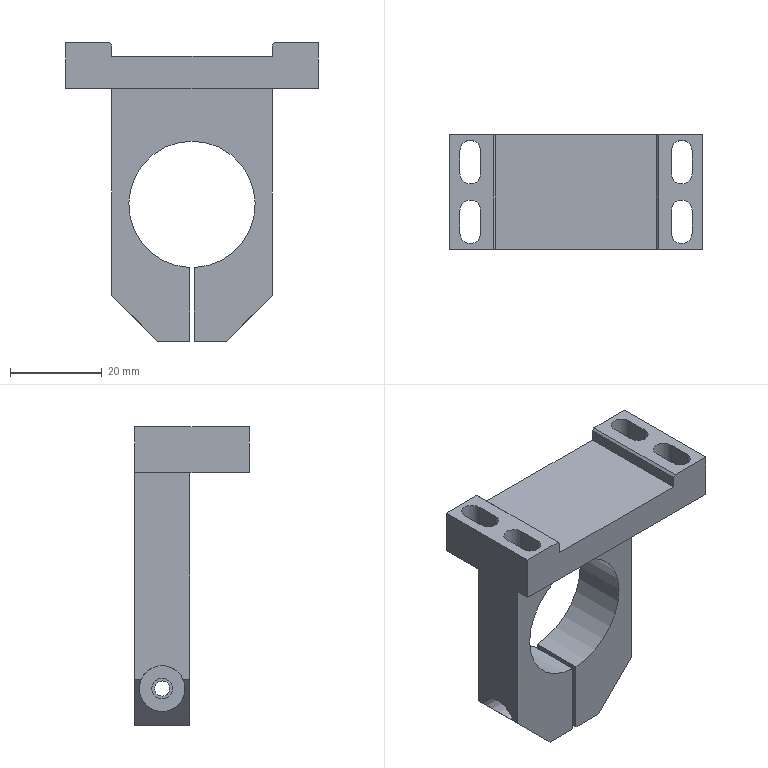Part | SolidWorks | features ICE 6, Chamfer 2, Extrusion 1, HoleWzd 1 | 1 solid | 45 faces | box 55 x 25 x 65 mm | volume 23319 mm3 | plane 30 | cylinder 15 | commonest cylinder face diameters 4.5 x10 3.3 x2 10 x2 27.5 x1
STEP:
#1=CARTESIAN_POINT('',(17.15,6.,-20.15));
#2=VERTEX_POINT('',#1);
#3=CARTESIAN_POINT('',(13.85,6.,-23.45));
#4=VERTEX_POINT('',#3);
#5=CARTESIAN_POINT('',(17.15,6.,-20.15));
#6=CARTESIAN_POINT('',(17.15,2.7,-20.15));
#7=CARTESIAN_POINT('',(13.85,2.7,-23.45));
#8=CARTESIAN_POINT('',(13.85,6.,-23.45));
#9=(BOUNDED_CURVE()B_SPLINE_CURVE(3,(#5,#6,#7,#8),.UNSPECIFIED.,.F.,.F.)B_SPLINE_CURVE_WITH_KNOTS((4,4),(3.142,6.283),.UNSPECIFIED.)CURVE()GEOMETRIC_REPRESENTATION_ITEM()RATIONAL_B_SPLINE_CURVE((1.,0.3333,0.3333,1.))REPRESENTATION_ITEM(''));
#10=EDGE_CURVE('',#2,#4,#9,.T.);
#11=ORIENTED_EDGE('',*,*,#10,.T.);
#12=CARTESIAN_POINT('',(0.5,6.,-23.45));
#13=VERTEX_POINT('',#12);
#14=CARTESIAN_POINT('',(0.5,6.,-23.45));
#15=DIRECTION('',(-1.,0.,0.));
#16=VECTOR('',#15,1000.);
#17=LINE('',#14,#16);
#18=EDGE_CURVE('',#4,#13,#17,.T.);
#19=ORIENTED_EDGE('',*,*,#18,.T.);
#20=CARTESIAN_POINT('',(0.5,6.,-20.15));
#21=VERTEX_POINT('',#20);
#22=CARTESIAN_POINT('',(0.5,6.,-21.8));
#23=DIRECTION('',(-1.,0.,0.));
#24=DIRECTION('',(0.,0.,1.));
#25=AXIS2_PLACEMENT_3D('',#22,#23,#24);
#26=CIRCLE('',#25,1.65);
#27=EDGE_CURVE('',#13,#21,#26,.T.);
#28=ORIENTED_EDGE('',*,*,#27,.T.);
#29=CARTESIAN_POINT('',(0.5,6.,-20.15));
#30=DIRECTION('',(-1.,0.,0.));
#31=VECTOR('',#30,1000.);
#32=LINE('',#29,#31);
#33=EDGE_CURVE('',#2,#21,#32,.T.);
#34=ORIENTED_EDGE('',*,*,#33,.F.);
#35=EDGE_LOOP('',(#11,#19,#28,#34));
#36=FACE_OUTER_BOUND('',#35,.T.);
#37=CARTESIAN_POINT('',(0.5,6.,-21.8));
#38=DIRECTION('',(-1.,0.,0.));
#39=DIRECTION('',(0.,0.,1.));
#40=AXIS2_PLACEMENT_3D('',#37,#38,#39);
#41=CYLINDRICAL_SURFACE('',#40,1.65);
#42=ADVANCED_FACE('',(#36),#41,.F.);
#43=CARTESIAN_POINT('',(-0.5,6.,-19.55));
#44=VERTEX_POINT('',#43);
#45=CARTESIAN_POINT('',(-0.5,6.,-24.05));
#46=VERTEX_POINT('',#45);
#47=CARTESIAN_POINT('',(-0.5,6.,-21.8));
#48=DIRECTION('',(1.,0.,0.));
#49=DIRECTION('',(0.,0.,1.));
#50=AXIS2_PLACEMENT_3D('',#47,#48,#49);
#51=CIRCLE('',#50,2.25);
#52=EDGE_CURVE('',#44,#46,#51,.T.);
#53=ORIENTED_EDGE('',*,*,#52,.T.);
#54=CARTESIAN_POINT('',(-7.5,6.,-24.05));
#55=VERTEX_POINT('',#54);
#56=CARTESIAN_POINT('',(5.864,6.,-24.05));
#57=DIRECTION('',(-1.,0.,0.));
#58=VECTOR('',#57,1000.);
#59=LINE('',#56,#58);
#60=EDGE_CURVE('',#46,#55,#59,.T.);
#61=ORIENTED_EDGE('',*,*,#60,.T.);
#62=CARTESIAN_POINT('',(-7.5,6.,-19.55));
#63=VERTEX_POINT('',#62);
#64=CARTESIAN_POINT('',(-7.5,6.,-21.8));
#65=DIRECTION('',(-1.,0.,0.));
#66=DIRECTION('',(0.,0.,1.));
#67=AXIS2_PLACEMENT_3D('',#64,#65,#66);
#68=CIRCLE('',#67,2.25);
#69=EDGE_CURVE('',#55,#63,#68,.T.);
#70=ORIENTED_EDGE('',*,*,#69,.T.);
#71=CARTESIAN_POINT('',(5.864,6.,-19.55));
#72=DIRECTION('',(-1.,0.,0.));
#73=VECTOR('',#72,1000.);
#74=LINE('',#71,#73);
#75=EDGE_CURVE('',#44,#63,#74,.T.);
#76=ORIENTED_EDGE('',*,*,#75,.F.);
#77=EDGE_LOOP('',(#53,#61,#70,#76));
#78=FACE_OUTER_BOUND('',#77,.T.);
#79=CARTESIAN_POINT('',(5.864,6.,-21.8));
#80=DIRECTION('',(-1.,0.,0.));
#81=DIRECTION('',(0.,0.,1.));
#82=AXIS2_PLACEMENT_3D('',#79,#80,#81);
#83=CYLINDRICAL_SURFACE('',#82,2.25);
#84=ADVANCED_FACE('',(#78),#83,.F.);
#85=CARTESIAN_POINT('',(-7.5,6.,-26.8));
#86=VERTEX_POINT('',#85);
#87=CARTESIAN_POINT('',(-7.5,6.,-16.8));
#88=VERTEX_POINT('',#87);
#89=CARTESIAN_POINT('',(-7.5,6.,-21.8));
#90=DIRECTION('',(-1.,0.,0.));
#91=DIRECTION('',(0.,0.,1.));
#92=AXIS2_PLACEMENT_3D('',#89,#90,#91);
#93=CIRCLE('',#92,5.);
#94=EDGE_CURVE('',#86,#88,#93,.T.);
#95=ORIENTED_EDGE('',*,*,#94,.F.);
#96=CARTESIAN_POINT('',(-10.5,6.,-26.8));
#97=VERTEX_POINT('',#96);
#98=CARTESIAN_POINT('',(-7.5,6.,-26.8));
#99=DIRECTION('',(-1.,0.,0.));
#100=VECTOR('',#99,1000.);
#101=LINE('',#98,#100);
#102=EDGE_CURVE('',#86,#97,#101,.T.);
#103=ORIENTED_EDGE('',*,*,#102,.T.);
#104=CARTESIAN_POINT('',(-17.5,1.417,-19.8));
#105=VERTEX_POINT('',#104);
#106=CARTESIAN_POINT('',(-10.5,6.,-26.8));
#107=CARTESIAN_POINT('',(-10.5,2.007,-26.8));
#108=CARTESIAN_POINT('',(-13.841,-0.1797,-23.459));
#109=CARTESIAN_POINT('',(-17.5,1.417,-19.8));
#110=(BOUNDED_CURVE()B_SPLINE_CURVE(3,(#106,#107,#108,#109),.UNSPECIFIED.,.F.,.F.)B_SPLINE_CURVE_WITH_KNOTS((4,4),(3.142,5.124),.UNSPECIFIED.)CURVE()GEOMETRIC_REPRESENTATION_ITEM()RATIONAL_B_SPLINE_CURVE((1.,0.6985,0.6985,1.))REPRESENTATION_ITEM(''));
#111=EDGE_CURVE('',#97,#105,#110,.T.);
#112=ORIENTED_EDGE('',*,*,#111,.T.);
#113=CARTESIAN_POINT('',(-17.5,6.,-16.8));
#114=VERTEX_POINT('',#113);
#115=CARTESIAN_POINT('',(-17.5,6.,-21.8));
#116=DIRECTION('',(-1.,0.,0.));
#117=DIRECTION('',(0.,0.,1.));
#118=AXIS2_PLACEMENT_3D('',#115,#116,#117);
#119=CIRCLE('',#118,5.);
#120=EDGE_CURVE('',#105,#114,#119,.T.);
#121=ORIENTED_EDGE('',*,*,#120,.T.);
#122=CARTESIAN_POINT('',(-7.5,6.,-16.8));
#123=DIRECTION('',(-1.,0.,0.));
#124=VECTOR('',#123,1000.);
#125=LINE('',#122,#124);
#126=EDGE_CURVE('',#88,#114,#125,.T.);
#127=ORIENTED_EDGE('',*,*,#126,.F.);
#128=EDGE_LOOP('',(#95,#103,#112,#121,#127));
#129=FACE_OUTER_BOUND('',#128,.T.);
#130=CARTESIAN_POINT('',(-7.5,6.,-21.8));
#131=DIRECTION('',(-1.,0.,0.));
#132=DIRECTION('',(0.,0.,1.));
#133=AXIS2_PLACEMENT_3D('',#130,#131,#132);
#134=CYLINDRICAL_SURFACE('',#133,5.);
#135=ADVANCED_FACE('',(#129),#134,.F.);
#136=CARTESIAN_POINT('',(7.5,0.,-29.8));
#137=VERTEX_POINT('',#136);
#138=CARTESIAN_POINT('',(0.5,0.,-29.8));
#139=VERTEX_POINT('',#138);
#140=CARTESIAN_POINT('',(-17.5,0.,-29.8));
#141=DIRECTION('',(-1.,0.,0.));
#142=VECTOR('',#141,1000.);
#143=LINE('',#140,#142);
#144=EDGE_CURVE('',#137,#139,#143,.T.);
#145=ORIENTED_EDGE('',*,*,#144,.T.);
#146=CARTESIAN_POINT('',(0.5,12.,-29.8));
#147=VERTEX_POINT('',#146);
#148=CARTESIAN_POINT('',(0.5,12.,-29.8));
#149=DIRECTION('',(0.,1.,0.));
#150=VECTOR('',#149,1000.);
#151=LINE('',#148,#150);
#152=EDGE_CURVE('',#139,#147,#151,.T.);
#153=ORIENTED_EDGE('',*,*,#152,.T.);
#154=CARTESIAN_POINT('',(7.5,12.,-29.8));
#155=VERTEX_POINT('',#154);
#156=CARTESIAN_POINT('',(-17.5,12.,-29.8));
#157=DIRECTION('',(-1.,0.,0.));
#158=VECTOR('',#157,1000.);
#159=LINE('',#156,#158);
#160=EDGE_CURVE('',#155,#147,#159,.T.);
#161=ORIENTED_EDGE('',*,*,#160,.F.);
#162=CARTESIAN_POINT('',(7.5,12.,-29.8));
#163=DIRECTION('',(0.,-1.,0.));
#164=VECTOR('',#163,1000.);
#165=LINE('',#162,#164);
#166=EDGE_CURVE('',#155,#137,#165,.T.);
#167=ORIENTED_EDGE('',*,*,#166,.T.);
#168=EDGE_LOOP('',(#145,#153,#161,#167));
#169=FACE_OUTER_BOUND('',#168,.T.);
#170=CARTESIAN_POINT('',(-17.5,12.,-29.8));
#171=DIRECTION('',(0.,0.,1.));
#172=DIRECTION('',(1.,0.,0.));
#173=AXIS2_PLACEMENT_3D('',#170,#171,#172);
#174=PLANE('',#173);
#175=ADVANCED_FACE('',(#169),#174,.F.);
#176=CARTESIAN_POINT('',(25.25,-4.5,35.2));
#177=VERTEX_POINT('',#176);
#178=CARTESIAN_POINT('',(25.25,-9.5,35.2));
#179=VERTEX_POINT('',#178);
#180=CARTESIAN_POINT('',(25.25,12.,35.2));
#181=DIRECTION('',(0.,-1.,0.));
#182=VECTOR('',#181,1000.);
#183=LINE('',#180,#182);
#184=EDGE_CURVE('',#177,#179,#183,.T.);
#185=ORIENTED_EDGE('',*,*,#184,.T.);
#186=CARTESIAN_POINT('',(20.75,-9.5,35.2));
#187=VERTEX_POINT('',#186);
#188=CARTESIAN_POINT('',(23.,-9.5,35.2));
#189=DIRECTION('',(0.,0.,-1.));
#190=DIRECTION('',(-1.,0.,0.));
#191=AXIS2_PLACEMENT_3D('',#188,#189,#190);
#192=CIRCLE('',#191,2.25);
#193=EDGE_CURVE('',#179,#187,#192,.T.);
#194=ORIENTED_EDGE('',*,*,#193,.T.);
#195=CARTESIAN_POINT('',(20.75,-4.5,35.2));
#196=VERTEX_POINT('',#195);
#197=CARTESIAN_POINT('',(20.75,12.,35.2));
#198=DIRECTION('',(0.,1.,0.));
#199=VECTOR('',#198,1000.);
#200=LINE('',#197,#199);
#201=EDGE_CURVE('',#187,#196,#200,.T.);
#202=ORIENTED_EDGE('',*,*,#201,.T.);
#203=CARTESIAN_POINT('',(23.,-4.5,35.2));
#204=DIRECTION('',(0.,0.,-1.));
#205=DIRECTION('',(-1.,0.,0.));
#206=AXIS2_PLACEMENT_3D('',#203,#204,#205);
#207=CIRCLE('',#206,2.25);
#208=EDGE_CURVE('',#196,#177,#207,.T.);
#209=ORIENTED_EDGE('',*,*,#208,.T.);
#210=EDGE_LOOP('',(#185,#194,#202,#209));
#211=FACE_BOUND('',#210,.T.);
#212=CARTESIAN_POINT('',(20.75,3.5,35.2));
#213=VERTEX_POINT('',#212);
#214=CARTESIAN_POINT('',(20.75,8.5,35.2));
#215=VERTEX_POINT('',#214);
#216=CARTESIAN_POINT('',(20.75,12.,35.2));
#217=DIRECTION('',(0.,1.,0.));
#218=VECTOR('',#217,1000.);
#219=LINE('',#216,#218);
#220=EDGE_CURVE('',#213,#215,#219,.T.);
#221=ORIENTED_EDGE('',*,*,#220,.T.);
#222=CARTESIAN_POINT('',(25.25,8.5,35.2));
#223=VERTEX_POINT('',#222);
#224=CARTESIAN_POINT('',(23.,8.5,35.2));
#225=DIRECTION('',(0.,0.,-1.));
#226=DIRECTION('',(-1.,0.,0.));
#227=AXIS2_PLACEMENT_3D('',#224,#225,#226);
#228=CIRCLE('',#227,2.25);
#229=EDGE_CURVE('',#215,#223,#228,.T.);
#230=ORIENTED_EDGE('',*,*,#229,.T.);
#231=CARTESIAN_POINT('',(25.25,3.5,35.2));
#232=VERTEX_POINT('',#231);
#233=CARTESIAN_POINT('',(25.25,12.,35.2));
#234=DIRECTION('',(0.,-1.,0.));
#235=VECTOR('',#234,1000.);
#236=LINE('',#233,#235);
#237=EDGE_CURVE('',#223,#232,#236,.T.);
#238=ORIENTED_EDGE('',*,*,#237,.T.);
#239=CARTESIAN_POINT('',(23.,3.5,35.2));
#240=DIRECTION('',(0.,0.,-1.));
#241=DIRECTION('',(-1.,0.,0.));
#242=AXIS2_PLACEMENT_3D('',#239,#240,#241);
#243=CIRCLE('',#242,2.25);
#244=EDGE_CURVE('',#232,#213,#243,.T.);
#245=ORIENTED_EDGE('',*,*,#244,.T.);
#246=EDGE_LOOP('',(#221,#230,#238,#245));
#247=FACE_BOUND('',#246,.T.);
#248=CARTESIAN_POINT('',(18.,12.,35.2));
#249=VERTEX_POINT('',#248);
#250=CARTESIAN_POINT('',(27.5,12.,35.2));
#251=VERTEX_POINT('',#250);
#252=CARTESIAN_POINT('',(-17.5,12.,35.2));
#253=DIRECTION('',(1.,0.,0.));
#254=VECTOR('',#253,1000.);
#255=LINE('',#252,#254);
#256=EDGE_CURVE('',#249,#251,#255,.T.);
#257=ORIENTED_EDGE('',*,*,#256,.F.);
#258=CARTESIAN_POINT('',(18.,-13.,35.2));
#259=VERTEX_POINT('',#258);
#260=CARTESIAN_POINT('',(18.,12.,35.2));
#261=DIRECTION('',(0.,-1.,0.));
#262=VECTOR('',#261,1000.);
#263=LINE('',#260,#262);
#264=EDGE_CURVE('',#249,#259,#263,.T.);
#265=ORIENTED_EDGE('',*,*,#264,.T.);
#266=CARTESIAN_POINT('',(27.5,-13.,35.2));
#267=VERTEX_POINT('',#266);
#268=CARTESIAN_POINT('',(-27.5,-13.,35.2));
#269=DIRECTION('',(1.,0.,0.));
#270=VECTOR('',#269,1000.);
#271=LINE('',#268,#270);
#272=EDGE_CURVE('',#259,#267,#271,.T.);
#273=ORIENTED_EDGE('',*,*,#272,.T.);
#274=CARTESIAN_POINT('',(27.5,-13.,35.2));
#275=DIRECTION('',(0.,1.,0.));
#276=VECTOR('',#275,1000.);
#277=LINE('',#274,#276);
#278=EDGE_CURVE('',#267,#251,#277,.T.);
#279=ORIENTED_EDGE('',*,*,#278,.T.);
#280=EDGE_LOOP('',(#257,#265,#273,#279));
#281=FACE_OUTER_BOUND('',#280,.T.);
#282=CARTESIAN_POINT('',(-17.5,12.,35.2));
#283=DIRECTION('',(0.,0.,-1.));
#284=DIRECTION('',(-1.,0.,0.));
#285=AXIS2_PLACEMENT_3D('',#282,#283,#284);
#286=PLANE('',#285);
#287=ADVANCED_FACE('',(#211,#247,#281),#286,.F.);
#288=ORIENTED_EDGE('',*,*,#160,.T.);
#289=CARTESIAN_POINT('',(0.5,12.,-13.741));
#290=VERTEX_POINT('',#289);
#291=CARTESIAN_POINT('',(0.5,12.,-48.692));
#292=DIRECTION('',(0.,0.,-1.));
#293=VECTOR('',#292,1000.);
#294=LINE('',#291,#293);
#295=EDGE_CURVE('',#290,#147,#294,.T.);
#296=ORIENTED_EDGE('',*,*,#295,.F.);
#297=CARTESIAN_POINT('',(-0.5,12.,-13.741));
#298=VERTEX_POINT('',#297);
#299=CARTESIAN_POINT('',(0.,12.,0.));
#300=DIRECTION('',(0.,1.,0.));
#301=DIRECTION('',(0.,0.,1.));
#302=AXIS2_PLACEMENT_3D('',#299,#300,#301);
#303=CIRCLE('',#302,13.75);
#304=EDGE_CURVE('',#298,#290,#303,.T.);
#305=ORIENTED_EDGE('',*,*,#304,.F.);
#306=CARTESIAN_POINT('',(-0.5,12.,-29.8));
#307=VERTEX_POINT('',#306);
#308=CARTESIAN_POINT('',(-0.5,12.,-48.692));
#309=DIRECTION('',(0.,0.,1.));
#310=VECTOR('',#309,1000.);
#311=LINE('',#308,#310);
#312=EDGE_CURVE('',#307,#298,#311,.T.);
#313=ORIENTED_EDGE('',*,*,#312,.F.);
#314=CARTESIAN_POINT('',(-7.5,12.,-29.8));
#315=VERTEX_POINT('',#314);
#316=CARTESIAN_POINT('',(-17.5,12.,-29.8));
#317=DIRECTION('',(-1.,0.,0.));
#318=VECTOR('',#317,1000.);
#319=LINE('',#316,#318);
#320=EDGE_CURVE('',#307,#315,#319,.T.);
#321=ORIENTED_EDGE('',*,*,#320,.T.);
#322=CARTESIAN_POINT('',(-17.5,12.,-19.8));
#323=VERTEX_POINT('',#322);
#324=CARTESIAN_POINT('',(-17.5,12.,-19.8));
#325=DIRECTION('',(-0.7071,0.,0.7071));
#326=VECTOR('',#325,1000.);
#327=LINE('',#324,#326);
#328=EDGE_CURVE('',#315,#323,#327,.T.);
#329=ORIENTED_EDGE('',*,*,#328,.T.);
#330=CARTESIAN_POINT('',(-17.5,12.,25.2));
#331=VERTEX_POINT('',#330);
#332=CARTESIAN_POINT('',(-17.5,12.,35.2));
#333=DIRECTION('',(0.,0.,1.));
#334=VECTOR('',#333,1000.);
#335=LINE('',#332,#334);
#336=EDGE_CURVE('',#323,#331,#335,.T.);
#337=ORIENTED_EDGE('',*,*,#336,.T.);
#338=CARTESIAN_POINT('',(-27.5,12.,25.2));
#339=VERTEX_POINT('',#338);
#340=CARTESIAN_POINT('',(-27.5,12.,25.2));
#341=DIRECTION('',(-1.,0.,0.));
#342=VECTOR('',#341,1000.);
#343=LINE('',#340,#342);
#344=EDGE_CURVE('',#331,#339,#343,.T.);
#345=ORIENTED_EDGE('',*,*,#344,.T.);
#346=CARTESIAN_POINT('',(-27.5,12.,35.2));
#347=VERTEX_POINT('',#346);
#348=CARTESIAN_POINT('',(-27.5,12.,25.2));
#349=DIRECTION('',(0.,0.,1.));
#350=VECTOR('',#349,1000.);
#351=LINE('',#348,#350);
#352=EDGE_CURVE('',#339,#347,#351,.T.);
#353=ORIENTED_EDGE('',*,*,#352,.T.);
#354=CARTESIAN_POINT('',(-18.,12.,35.2));
#355=VERTEX_POINT('',#354);
#356=CARTESIAN_POINT('',(-17.5,12.,35.2));
#357=DIRECTION('',(1.,0.,0.));
#358=VECTOR('',#357,1000.);
#359=LINE('',#356,#358);
#360=EDGE_CURVE('',#347,#355,#359,.T.);
#361=ORIENTED_EDGE('',*,*,#360,.T.);
#362=CARTESIAN_POINT('',(-17.5,12.,34.7));
#363=VERTEX_POINT('',#362);
#364=CARTESIAN_POINT('',(-18.,12.,35.2));
#365=DIRECTION('',(0.7071,0.,-0.7071));
#366=VECTOR('',#365,1000.);
#367=LINE('',#364,#366);
#368=EDGE_CURVE('',#355,#363,#367,.T.);
#369=ORIENTED_EDGE('',*,*,#368,.T.);
#370=CARTESIAN_POINT('',(-17.5,12.,32.2));
#371=VERTEX_POINT('',#370);
#372=CARTESIAN_POINT('',(-17.5,12.,38.2));
#373=DIRECTION('',(0.,0.,-1.));
#374=VECTOR('',#373,1000.);
#375=LINE('',#372,#374);
#376=EDGE_CURVE('',#363,#371,#375,.T.);
#377=ORIENTED_EDGE('',*,*,#376,.T.);
#378=CARTESIAN_POINT('',(17.5,12.,32.2));
#379=VERTEX_POINT('',#378);
#380=CARTESIAN_POINT('',(-17.5,12.,32.2));
#381=DIRECTION('',(1.,0.,0.));
#382=VECTOR('',#381,1000.);
#383=LINE('',#380,#382);
#384=EDGE_CURVE('',#371,#379,#383,.T.);
#385=ORIENTED_EDGE('',*,*,#384,.T.);
#386=CARTESIAN_POINT('',(17.5,12.,34.7));
#387=VERTEX_POINT('',#386);
#388=CARTESIAN_POINT('',(17.5,12.,38.2));
#389=DIRECTION('',(0.,0.,1.));
#390=VECTOR('',#389,1000.);
#391=LINE('',#388,#390);
#392=EDGE_CURVE('',#379,#387,#391,.T.);
#393=ORIENTED_EDGE('',*,*,#392,.T.);
#394=CARTESIAN_POINT('',(18.,12.,35.2));
#395=DIRECTION('',(0.7071,0.,0.7071));
#396=VECTOR('',#395,1000.);
#397=LINE('',#394,#396);
#398=EDGE_CURVE('',#387,#249,#397,.T.);
#399=ORIENTED_EDGE('',*,*,#398,.T.);
#400=ORIENTED_EDGE('',*,*,#256,.T.);
#401=CARTESIAN_POINT('',(27.5,12.,25.2));
#402=VERTEX_POINT('',#401);
#403=CARTESIAN_POINT('',(27.5,12.,25.2));
#404=DIRECTION('',(0.,0.,-1.));
#405=VECTOR('',#404,1000.);
#406=LINE('',#403,#405);
#407=EDGE_CURVE('',#251,#402,#406,.T.);
#408=ORIENTED_EDGE('',*,*,#407,.T.);
#409=CARTESIAN_POINT('',(17.5,12.,25.2));
#410=VERTEX_POINT('',#409);
#411=CARTESIAN_POINT('',(-27.5,12.,25.2));
#412=DIRECTION('',(-1.,0.,0.));
#413=VECTOR('',#412,1000.);
#414=LINE('',#411,#413);
#415=EDGE_CURVE('',#402,#410,#414,.T.);
#416=ORIENTED_EDGE('',*,*,#415,.T.);
#417=CARTESIAN_POINT('',(17.5,12.,-19.8));
#418=VERTEX_POINT('',#417);
#419=CARTESIAN_POINT('',(17.5,12.,35.2));
#420=DIRECTION('',(0.,0.,-1.));
#421=VECTOR('',#420,1000.);
#422=LINE('',#419,#421);
#423=EDGE_CURVE('',#410,#418,#422,.T.);
#424=ORIENTED_EDGE('',*,*,#423,.T.);
#425=CARTESIAN_POINT('',(7.5,12.,-29.8));
#426=DIRECTION('',(-0.7071,0.,-0.7071));
#427=VECTOR('',#426,1000.);
#428=LINE('',#425,#427);
#429=EDGE_CURVE('',#418,#155,#428,.T.);
#430=ORIENTED_EDGE('',*,*,#429,.T.);
#431=EDGE_LOOP('',(#288,#296,#305,#313,#321,#329,#337,#345,#353,#361,#369,#377,#385,#393,#399,#400,#408,#416,#424,#430));
#432=FACE_OUTER_BOUND('',#431,.T.);
#433=CARTESIAN_POINT('',(0.,12.,0.));
#434=DIRECTION('',(0.,-1.,0.));
#435=DIRECTION('',(0.,0.,-1.));
#436=AXIS2_PLACEMENT_3D('',#433,#434,#435);
#437=PLANE('',#436);
#438=ADVANCED_FACE('',(#432),#437,.F.);
#439=CARTESIAN_POINT('',(0.5,0.,-13.741));
#440=VERTEX_POINT('',#439);
#441=CARTESIAN_POINT('',(0.5,0.,0.));
#442=DIRECTION('',(0.,0.,1.));
#443=VECTOR('',#442,1000.);
#444=LINE('',#441,#443);
#445=EDGE_CURVE('',#139,#440,#444,.T.);
#446=ORIENTED_EDGE('',*,*,#445,.F.);
#447=ORIENTED_EDGE('',*,*,#144,.F.);
#448=CARTESIAN_POINT('',(17.5,0.,-19.8));
#449=VERTEX_POINT('',#448);
#450=CARTESIAN_POINT('',(18.65,0.,-18.65));
#451=DIRECTION('',(0.7071,0.,0.7071));
#452=VECTOR('',#451,1000.);
#453=LINE('',#450,#452);
#454=EDGE_CURVE('',#137,#449,#453,.T.);
#455=ORIENTED_EDGE('',*,*,#454,.T.);
#456=CARTESIAN_POINT('',(17.5,0.,25.2));
#457=VERTEX_POINT('',#456);
#458=CARTESIAN_POINT('',(17.5,0.,35.2));
#459=DIRECTION('',(0.,0.,-1.));
#460=VECTOR('',#459,1000.);
#461=LINE('',#458,#460);
#462=EDGE_CURVE('',#457,#449,#461,.T.);
#463=ORIENTED_EDGE('',*,*,#462,.F.);
#464=CARTESIAN_POINT('',(-17.5,0.,25.2));
#465=VERTEX_POINT('',#464);
#466=CARTESIAN_POINT('',(0.,0.,25.2));
#467=DIRECTION('',(1.,0.,0.));
#468=VECTOR('',#467,1000.);
#469=LINE('',#466,#468);
#470=EDGE_CURVE('',#465,#457,#469,.T.);
#471=ORIENTED_EDGE('',*,*,#470,.F.);
#472=CARTESIAN_POINT('',(-17.5,0.,-19.8));
#473=VERTEX_POINT('',#472);
#474=CARTESIAN_POINT('',(-17.5,0.,35.2));
#475=DIRECTION('',(0.,0.,1.));
#476=VECTOR('',#475,1000.);
#477=LINE('',#474,#476);
#478=EDGE_CURVE('',#473,#465,#477,.T.);
#479=ORIENTED_EDGE('',*,*,#478,.F.);
#480=CARTESIAN_POINT('',(-7.5,0.,-29.8));
#481=VERTEX_POINT('',#480);
#482=CARTESIAN_POINT('',(-18.65,0.,-18.65));
#483=DIRECTION('',(0.7071,0.,-0.7071));
#484=VECTOR('',#483,1000.);
#485=LINE('',#482,#484);
#486=EDGE_CURVE('',#473,#481,#485,.T.);
#487=ORIENTED_EDGE('',*,*,#486,.T.);
#488=CARTESIAN_POINT('',(-0.5,0.,-29.8));
#489=VERTEX_POINT('',#488);
#490=CARTESIAN_POINT('',(-17.5,0.,-29.8));
#491=DIRECTION('',(-1.,0.,0.));
#492=VECTOR('',#491,1000.);
#493=LINE('',#490,#492);
#494=EDGE_CURVE('',#489,#481,#493,.T.);
#495=ORIENTED_EDGE('',*,*,#494,.F.);
#496=CARTESIAN_POINT('',(-0.5,0.,-13.741));
#497=VERTEX_POINT('',#496);
#498=CARTESIAN_POINT('',(-0.5,0.,0.));
#499=DIRECTION('',(0.,0.,-1.));
#500=VECTOR('',#499,1000.);
#501=LINE('',#498,#500);
#502=EDGE_CURVE('',#497,#489,#501,.T.);
#503=ORIENTED_EDGE('',*,*,#502,.F.);
#504=CARTESIAN_POINT('',(0.,0.,0.));
#505=DIRECTION('',(0.,1.,0.));
#506=DIRECTION('',(0.,0.,1.));
#507=AXIS2_PLACEMENT_3D('',#504,#505,#506);
#508=CIRCLE('',#507,13.75);
#509=EDGE_CURVE('',#497,#440,#508,.T.);
#510=ORIENTED_EDGE('',*,*,#509,.T.);
#511=EDGE_LOOP('',(#446,#447,#455,#463,#471,#479,#487,#495,#503,#510));
#512=FACE_OUTER_BOUND('',#511,.T.);
#513=CARTESIAN_POINT('',(0.,0.,0.));
#514=DIRECTION('',(0.,-1.,0.));
#515=DIRECTION('',(0.,0.,-1.));
#516=AXIS2_PLACEMENT_3D('',#513,#514,#515);
#517=PLANE('',#516);
#518=ADVANCED_FACE('',(#512),#517,.T.);
#519=ORIENTED_EDGE('',*,*,#423,.F.);
#520=CARTESIAN_POINT('',(17.5,12.,25.2));
#521=DIRECTION('',(0.,-1.,0.));
#522=VECTOR('',#521,1000.);
#523=LINE('',#520,#522);
#524=EDGE_CURVE('',#410,#457,#523,.T.);
#525=ORIENTED_EDGE('',*,*,#524,.T.);
#526=ORIENTED_EDGE('',*,*,#462,.T.);
#527=CARTESIAN_POINT('',(17.5,12.,-19.8));
#528=DIRECTION('',(0.,1.,0.));
#529=VECTOR('',#528,1000.);
#530=LINE('',#527,#529);
#531=EDGE_CURVE('',#449,#418,#530,.T.);
#532=ORIENTED_EDGE('',*,*,#531,.T.);
#533=EDGE_LOOP('',(#519,#525,#526,#532));
#534=FACE_OUTER_BOUND('',#533,.T.);
#535=CARTESIAN_POINT('',(17.5,12.,35.2));
#536=DIRECTION('',(-1.,0.,0.));
#537=DIRECTION('',(0.,0.,1.));
#538=AXIS2_PLACEMENT_3D('',#535,#536,#537);
#539=PLANE('',#538);
#540=ADVANCED_FACE('',(#534),#539,.F.);
#541=ORIENTED_EDGE('',*,*,#320,.F.);
#542=CARTESIAN_POINT('',(-0.5,12.,-29.8));
#543=DIRECTION('',(0.,-1.,0.));
#544=VECTOR('',#543,1000.);
#545=LINE('',#542,#544);
#546=EDGE_CURVE('',#307,#489,#545,.T.);
#547=ORIENTED_EDGE('',*,*,#546,.T.);
#548=ORIENTED_EDGE('',*,*,#494,.T.);
#549=CARTESIAN_POINT('',(-7.5,12.,-29.8));
#550=DIRECTION('',(0.,1.,0.));
#551=VECTOR('',#550,1000.);
#552=LINE('',#549,#551);
#553=EDGE_CURVE('',#481,#315,#552,.T.);
#554=ORIENTED_EDGE('',*,*,#553,.T.);
#555=EDGE_LOOP('',(#541,#547,#548,#554));
#556=FACE_OUTER_BOUND('',#555,.T.);
#557=CARTESIAN_POINT('',(-17.5,12.,-29.8));
#558=DIRECTION('',(0.,0.,1.));
#559=DIRECTION('',(1.,0.,0.));
#560=AXIS2_PLACEMENT_3D('',#557,#558,#559);
#561=PLANE('',#560);
#562=ADVANCED_FACE('',(#556),#561,.F.);
#563=CARTESIAN_POINT('',(-17.5,10.583,-19.8));
#564=VERTEX_POINT('',#563);
#565=CARTESIAN_POINT('',(-17.5,12.,-19.8));
#566=DIRECTION('',(0.,-1.,0.));
#567=VECTOR('',#566,1000.);
#568=LINE('',#565,#567);
#569=EDGE_CURVE('',#323,#564,#568,.T.);
#570=ORIENTED_EDGE('',*,*,#569,.T.);
#571=CARTESIAN_POINT('',(-17.5,6.,-21.8));
#572=DIRECTION('',(-1.,0.,0.));
#573=DIRECTION('',(0.,0.,1.));
#574=AXIS2_PLACEMENT_3D('',#571,#572,#573);
#575=CIRCLE('',#574,5.);
#576=EDGE_CURVE('',#114,#564,#575,.T.);
#577=ORIENTED_EDGE('',*,*,#576,.F.);
#578=ORIENTED_EDGE('',*,*,#120,.F.);
#579=CARTESIAN_POINT('',(-17.5,12.,-19.8));
#580=DIRECTION('',(0.,-1.,0.));
#581=VECTOR('',#580,1000.);
#582=LINE('',#579,#581);
#583=EDGE_CURVE('',#105,#473,#582,.T.);
#584=ORIENTED_EDGE('',*,*,#583,.T.);
#585=ORIENTED_EDGE('',*,*,#478,.T.);
#586=CARTESIAN_POINT('',(-17.5,12.,25.2));
#587=DIRECTION('',(0.,1.,0.));
#588=VECTOR('',#587,1000.);
#589=LINE('',#586,#588);
#590=EDGE_CURVE('',#465,#331,#589,.T.);
#591=ORIENTED_EDGE('',*,*,#590,.T.);
#592=ORIENTED_EDGE('',*,*,#336,.F.);
#593=EDGE_LOOP('',(#570,#577,#578,#584,#585,#591,#592));
#594=FACE_OUTER_BOUND('',#593,.T.);
#595=CARTESIAN_POINT('',(-17.5,12.,35.2));
#596=DIRECTION('',(1.,0.,0.));
#597=DIRECTION('',(0.,0.,-1.));
#598=AXIS2_PLACEMENT_3D('',#595,#596,#597);
#599=PLANE('',#598);
#600=ADVANCED_FACE('',(#594),#599,.F.);
#601=CARTESIAN_POINT('',(-20.75,-4.5,35.2));
#602=VERTEX_POINT('',#601);
#603=CARTESIAN_POINT('',(-20.75,-9.5,35.2));
#604=VERTEX_POINT('',#603);
#605=CARTESIAN_POINT('',(-20.75,12.,35.2));
#606=DIRECTION('',(0.,-1.,0.));
#607=VECTOR('',#606,1000.);
#608=LINE('',#605,#607);
#609=EDGE_CURVE('',#602,#604,#608,.T.);
#610=ORIENTED_EDGE('',*,*,#609,.T.);
#611=CARTESIAN_POINT('',(-25.25,-9.5,35.2));
#612=VERTEX_POINT('',#611);
#613=CARTESIAN_POINT('',(-23.,-9.5,35.2));
#614=DIRECTION('',(0.,0.,-1.));
#615=DIRECTION('',(-1.,0.,0.));
#616=AXIS2_PLACEMENT_3D('',#613,#614,#615);
#617=CIRCLE('',#616,2.25);
#618=EDGE_CURVE('',#604,#612,#617,.T.);
#619=ORIENTED_EDGE('',*,*,#618,.T.);
#620=CARTESIAN_POINT('',(-25.25,-4.5,35.2));
#621=VERTEX_POINT('',#620);
#622=CARTESIAN_POINT('',(-25.25,12.,35.2));
#623=DIRECTION('',(0.,1.,0.));
#624=VECTOR('',#623,1000.);
#625=LINE('',#622,#624);
#626=EDGE_CURVE('',#612,#621,#625,.T.);
#627=ORIENTED_EDGE('',*,*,#626,.T.);
#628=CARTESIAN_POINT('',(-23.,-4.5,35.2));
#629=DIRECTION('',(0.,0.,-1.));
#630=DIRECTION('',(-1.,0.,0.));
#631=AXIS2_PLACEMENT_3D('',#628,#629,#630);
#632=CIRCLE('',#631,2.25);
#633=EDGE_CURVE('',#621,#602,#632,.T.);
#634=ORIENTED_EDGE('',*,*,#633,.T.);
#635=EDGE_LOOP('',(#610,#619,#627,#634));
#636=FACE_BOUND('',#635,.T.);
#637=CARTESIAN_POINT('',(-25.25,3.5,35.2));
#638=VERTEX_POINT('',#637);
#639=CARTESIAN_POINT('',(-25.25,8.5,35.2));
#640=VERTEX_POINT('',#639);
#641=CARTESIAN_POINT('',(-25.25,12.,35.2));
#642=DIRECTION('',(0.,1.,0.));
#643=VECTOR('',#642,1000.);
#644=LINE('',#641,#643);
#645=EDGE_CURVE('',#638,#640,#644,.T.);
#646=ORIENTED_EDGE('',*,*,#645,.T.);
#647=CARTESIAN_POINT('',(-20.75,8.5,35.2));
#648=VERTEX_POINT('',#647);
#649=CARTESIAN_POINT('',(-23.,8.5,35.2));
#650=DIRECTION('',(0.,0.,-1.));
#651=DIRECTION('',(-1.,0.,0.));
#652=AXIS2_PLACEMENT_3D('',#649,#650,#651);
#653=CIRCLE('',#652,2.25);
#654=EDGE_CURVE('',#640,#648,#653,.T.);
#655=ORIENTED_EDGE('',*,*,#654,.T.);
#656=CARTESIAN_POINT('',(-20.75,3.5,35.2));
#657=VERTEX_POINT('',#656);
#658=CARTESIAN_POINT('',(-20.75,12.,35.2));
#659=DIRECTION('',(0.,-1.,0.));
#660=VECTOR('',#659,1000.);
#661=LINE('',#658,#660);
#662=EDGE_CURVE('',#648,#657,#661,.T.);
#663=ORIENTED_EDGE('',*,*,#662,.T.);
#664=CARTESIAN_POINT('',(-23.,3.5,35.2));
#665=DIRECTION('',(0.,0.,-1.));
#666=DIRECTION('',(-1.,0.,0.));
#667=AXIS2_PLACEMENT_3D('',#664,#665,#666);
#668=CIRCLE('',#667,2.25);
#669=EDGE_CURVE('',#657,#638,#668,.T.);
#670=ORIENTED_EDGE('',*,*,#669,.T.);
#671=EDGE_LOOP('',(#646,#655,#663,#670));
#672=FACE_BOUND('',#671,.T.);
#673=CARTESIAN_POINT('',(-27.5,-13.,35.2));
#674=VERTEX_POINT('',#673);
#675=CARTESIAN_POINT('',(-18.,-13.,35.2));
#676=VERTEX_POINT('',#675);
#677=CARTESIAN_POINT('',(-27.5,-13.,35.2));
#678=DIRECTION('',(1.,0.,0.));
#679=VECTOR('',#678,1000.);
#680=LINE('',#677,#679);
#681=EDGE_CURVE('',#674,#676,#680,.T.);
#682=ORIENTED_EDGE('',*,*,#681,.T.);
#683=CARTESIAN_POINT('',(-18.,12.,35.2));
#684=DIRECTION('',(0.,1.,0.));
#685=VECTOR('',#684,1000.);
#686=LINE('',#683,#685);
#687=EDGE_CURVE('',#676,#355,#686,.T.);
#688=ORIENTED_EDGE('',*,*,#687,.T.);
#689=ORIENTED_EDGE('',*,*,#360,.F.);
#690=CARTESIAN_POINT('',(-27.5,-13.,35.2));
#691=DIRECTION('',(0.,1.,0.));
#692=VECTOR('',#691,1000.);
#693=LINE('',#690,#692);
#694=EDGE_CURVE('',#674,#347,#693,.T.);
#695=ORIENTED_EDGE('',*,*,#694,.F.);
#696=EDGE_LOOP('',(#682,#688,#689,#695));
#697=FACE_OUTER_BOUND('',#696,.T.);
#698=CARTESIAN_POINT('',(-17.5,12.,35.2));
#699=DIRECTION('',(0.,0.,-1.));
#700=DIRECTION('',(-1.,0.,0.));
#701=AXIS2_PLACEMENT_3D('',#698,#699,#700);
#702=PLANE('',#701);
#703=ADVANCED_FACE('',(#636,#672,#697),#702,.F.);
#704=CARTESIAN_POINT('',(0.5,12.,-13.741));
#705=DIRECTION('',(0.,1.,0.));
#706=VECTOR('',#705,1000.);
#707=LINE('',#704,#706);
#708=EDGE_CURVE('',#440,#290,#707,.T.);
#709=ORIENTED_EDGE('',*,*,#708,.F.);
#710=ORIENTED_EDGE('',*,*,#509,.F.);
#711=CARTESIAN_POINT('',(-0.5,12.,-13.741));
#712=DIRECTION('',(0.,-1.,0.));
#713=VECTOR('',#712,1000.);
#714=LINE('',#711,#713);
#715=EDGE_CURVE('',#298,#497,#714,.T.);
#716=ORIENTED_EDGE('',*,*,#715,.F.);
#717=ORIENTED_EDGE('',*,*,#304,.T.);
#718=EDGE_LOOP('',(#709,#710,#716,#717));
#719=FACE_OUTER_BOUND('',#718,.T.);
#720=CARTESIAN_POINT('',(0.,12.,0.));
#721=DIRECTION('',(0.,-1.,0.));
#722=DIRECTION('',(0.,0.,-1.));
#723=AXIS2_PLACEMENT_3D('',#720,#721,#722);
#724=CYLINDRICAL_SURFACE('',#723,13.75);
#725=ADVANCED_FACE('',(#719),#724,.F.);
#726=ORIENTED_EDGE('',*,*,#10,.F.);
#727=CARTESIAN_POINT('',(13.85,6.,-23.45));
#728=CARTESIAN_POINT('',(13.85,9.3,-23.45));
#729=CARTESIAN_POINT('',(17.15,9.3,-20.15));
#730=CARTESIAN_POINT('',(17.15,6.,-20.15));
#731=(BOUNDED_CURVE()B_SPLINE_CURVE(3,(#727,#728,#729,#730),.UNSPECIFIED.,.F.,.F.)B_SPLINE_CURVE_WITH_KNOTS((4,4),(0.,3.142),.UNSPECIFIED.)CURVE()GEOMETRIC_REPRESENTATION_ITEM()RATIONAL_B_SPLINE_CURVE((1.,0.3333,0.3333,1.))REPRESENTATION_ITEM(''));
#732=EDGE_CURVE('',#4,#2,#731,.T.);
#733=ORIENTED_EDGE('',*,*,#732,.F.);
#734=EDGE_LOOP('',(#726,#733));
#735=FACE_BOUND('',#734,.T.);
#736=ORIENTED_EDGE('',*,*,#429,.F.);
#737=ORIENTED_EDGE('',*,*,#531,.F.);
#738=ORIENTED_EDGE('',*,*,#454,.F.);
#739=ORIENTED_EDGE('',*,*,#166,.F.);
#740=EDGE_LOOP('',(#736,#737,#738,#739));
#741=FACE_OUTER_BOUND('',#740,.T.);
#742=CARTESIAN_POINT('',(7.5,12.,-29.8));
#743=DIRECTION('',(-0.7071,0.,0.7071));
#744=DIRECTION('',(0.,-1.,0.));
#745=AXIS2_PLACEMENT_3D('',#742,#743,#744);
#746=PLANE('',#745);
#747=ADVANCED_FACE('',(#735,#741),#746,.F.);
#748=CARTESIAN_POINT('',(-17.5,10.583,-19.8));
#749=CARTESIAN_POINT('',(-13.841,12.18,-23.459));
#750=CARTESIAN_POINT('',(-10.5,9.993,-26.8));
#751=CARTESIAN_POINT('',(-10.5,6.,-26.8));
#752=(BOUNDED_CURVE()B_SPLINE_CURVE(3,(#748,#749,#750,#751),.UNSPECIFIED.,.F.,.F.)B_SPLINE_CURVE_WITH_KNOTS((4,4),(1.159,3.142),.UNSPECIFIED.)CURVE()GEOMETRIC_REPRESENTATION_ITEM()RATIONAL_B_SPLINE_CURVE((1.,0.6985,0.6985,1.))REPRESENTATION_ITEM(''));
#753=EDGE_CURVE('',#564,#97,#752,.T.);
#754=ORIENTED_EDGE('',*,*,#753,.F.);
#755=ORIENTED_EDGE('',*,*,#569,.F.);
#756=ORIENTED_EDGE('',*,*,#328,.F.);
#757=ORIENTED_EDGE('',*,*,#553,.F.);
#758=ORIENTED_EDGE('',*,*,#486,.F.);
#759=ORIENTED_EDGE('',*,*,#583,.F.);
#760=ORIENTED_EDGE('',*,*,#111,.F.);
#761=EDGE_LOOP('',(#754,#755,#756,#757,#758,#759,#760));
#762=FACE_OUTER_BOUND('',#761,.T.);
#763=CARTESIAN_POINT('',(-17.5,12.,-19.8));
#764=DIRECTION('',(0.7071,0.,0.7071));
#765=DIRECTION('',(0.,-1.,0.));
#766=AXIS2_PLACEMENT_3D('',#763,#764,#765);
#767=PLANE('',#766);
#768=ADVANCED_FACE('',(#762),#767,.F.);
#769=CARTESIAN_POINT('',(25.25,-9.5,25.2));
#770=VERTEX_POINT('',#769);
#771=CARTESIAN_POINT('',(20.75,-9.5,25.2));
#772=VERTEX_POINT('',#771);
#773=CARTESIAN_POINT('',(23.,-9.5,25.2));
#774=DIRECTION('',(0.,0.,-1.));
#775=DIRECTION('',(1.,0.,0.));
#776=AXIS2_PLACEMENT_3D('',#773,#774,#775);
#777=CIRCLE('',#776,2.25);
#778=EDGE_CURVE('',#770,#772,#777,.T.);
#779=ORIENTED_EDGE('',*,*,#778,.F.);
#780=CARTESIAN_POINT('',(25.25,-4.5,25.2));
#781=VERTEX_POINT('',#780);
#782=CARTESIAN_POINT('',(25.25,-9.5,25.2));
#783=DIRECTION('',(0.,-1.,0.));
#784=VECTOR('',#783,1000.);
#785=LINE('',#782,#784);
#786=EDGE_CURVE('',#781,#770,#785,.T.);
#787=ORIENTED_EDGE('',*,*,#786,.F.);
#788=CARTESIAN_POINT('',(20.75,-4.5,25.2));
#789=VERTEX_POINT('',#788);
#790=CARTESIAN_POINT('',(23.,-4.5,25.2));
#791=DIRECTION('',(0.,0.,-1.));
#792=DIRECTION('',(1.,0.,0.));
#793=AXIS2_PLACEMENT_3D('',#790,#791,#792);
#794=CIRCLE('',#793,2.25);
#795=EDGE_CURVE('',#789,#781,#794,.T.);
#796=ORIENTED_EDGE('',*,*,#795,.F.);
#797=CARTESIAN_POINT('',(20.75,-9.5,25.2));
#798=DIRECTION('',(0.,1.,0.));
#799=VECTOR('',#798,1000.);
#800=LINE('',#797,#799);
#801=EDGE_CURVE('',#772,#789,#800,.T.);
#802=ORIENTED_EDGE('',*,*,#801,.F.);
#803=EDGE_LOOP('',(#779,#787,#796,#802));
#804=FACE_BOUND('',#803,.T.);
#805=CARTESIAN_POINT('',(-20.75,-9.5,25.2));
#806=VERTEX_POINT('',#805);
#807=CARTESIAN_POINT('',(-25.25,-9.5,25.2));
#808=VERTEX_POINT('',#807);
#809=CARTESIAN_POINT('',(-23.,-9.5,25.2));
#810=DIRECTION('',(0.,0.,-1.));
#811=DIRECTION('',(-1.,0.,0.));
#812=AXIS2_PLACEMENT_3D('',#809,#810,#811);
#813=CIRCLE('',#812,2.25);
#814=EDGE_CURVE('',#806,#808,#813,.T.);
#815=ORIENTED_EDGE('',*,*,#814,.F.);
#816=CARTESIAN_POINT('',(-20.75,-4.5,25.2));
#817=VERTEX_POINT('',#816);
#818=CARTESIAN_POINT('',(-20.75,-9.5,25.2));
#819=DIRECTION('',(0.,-1.,0.));
#820=VECTOR('',#819,1000.);
#821=LINE('',#818,#820);
#822=EDGE_CURVE('',#817,#806,#821,.T.);
#823=ORIENTED_EDGE('',*,*,#822,.F.);
#824=CARTESIAN_POINT('',(-25.25,-4.5,25.2));
#825=VERTEX_POINT('',#824);
#826=CARTESIAN_POINT('',(-23.,-4.5,25.2));
#827=DIRECTION('',(0.,0.,-1.));
#828=DIRECTION('',(-1.,0.,0.));
#829=AXIS2_PLACEMENT_3D('',#826,#827,#828);
#830=CIRCLE('',#829,2.25);
#831=EDGE_CURVE('',#825,#817,#830,.T.);
#832=ORIENTED_EDGE('',*,*,#831,.F.);
#833=CARTESIAN_POINT('',(-25.25,-9.5,25.2));
#834=DIRECTION('',(0.,1.,0.));
#835=VECTOR('',#834,1000.);
#836=LINE('',#833,#835);
#837=EDGE_CURVE('',#808,#825,#836,.T.);
#838=ORIENTED_EDGE('',*,*,#837,.F.);
#839=EDGE_LOOP('',(#815,#823,#832,#838));
#840=FACE_BOUND('',#839,.T.);
#841=CARTESIAN_POINT('',(-25.25,8.5,25.2));
#842=VERTEX_POINT('',#841);
#843=CARTESIAN_POINT('',(-20.75,8.5,25.2));
#844=VERTEX_POINT('',#843);
#845=CARTESIAN_POINT('',(-23.,8.5,25.2));
#846=DIRECTION('',(0.,0.,-1.));
#847=DIRECTION('',(1.,0.,0.));
#848=AXIS2_PLACEMENT_3D('',#845,#846,#847);
#849=CIRCLE('',#848,2.25);
#850=EDGE_CURVE('',#842,#844,#849,.T.);
#851=ORIENTED_EDGE('',*,*,#850,.F.);
#852=CARTESIAN_POINT('',(-25.25,3.5,25.2));
#853=VERTEX_POINT('',#852);
#854=CARTESIAN_POINT('',(-25.25,8.5,25.2));
#855=DIRECTION('',(0.,1.,0.));
#856=VECTOR('',#855,1000.);
#857=LINE('',#854,#856);
#858=EDGE_CURVE('',#853,#842,#857,.T.);
#859=ORIENTED_EDGE('',*,*,#858,.F.);
#860=CARTESIAN_POINT('',(-20.75,3.5,25.2));
#861=VERTEX_POINT('',#860);
#862=CARTESIAN_POINT('',(-23.,3.5,25.2));
#863=DIRECTION('',(0.,0.,-1.));
#864=DIRECTION('',(1.,0.,0.));
#865=AXIS2_PLACEMENT_3D('',#862,#863,#864);
#866=CIRCLE('',#865,2.25);
#867=EDGE_CURVE('',#861,#853,#866,.T.);
#868=ORIENTED_EDGE('',*,*,#867,.F.);
#869=CARTESIAN_POINT('',(-20.75,8.5,25.2));
#870=DIRECTION('',(0.,-1.,0.));
#871=VECTOR('',#870,1000.);
#872=LINE('',#869,#871);
#873=EDGE_CURVE('',#844,#861,#872,.T.);
#874=ORIENTED_EDGE('',*,*,#873,.F.);
#875=EDGE_LOOP('',(#851,#859,#868,#874));
#876=FACE_BOUND('',#875,.T.);
#877=CARTESIAN_POINT('',(20.75,8.5,25.2));
#878=VERTEX_POINT('',#877);
#879=CARTESIAN_POINT('',(25.25,8.5,25.2));
#880=VERTEX_POINT('',#879);
#881=CARTESIAN_POINT('',(23.,8.5,25.2));
#882=DIRECTION('',(0.,0.,-1.));
#883=DIRECTION('',(-1.,0.,0.));
#884=AXIS2_PLACEMENT_3D('',#881,#882,#883);
#885=CIRCLE('',#884,2.25);
#886=EDGE_CURVE('',#878,#880,#885,.T.);
#887=ORIENTED_EDGE('',*,*,#886,.F.);
#888=CARTESIAN_POINT('',(20.75,3.5,25.2));
#889=VERTEX_POINT('',#888);
#890=CARTESIAN_POINT('',(20.75,8.5,25.2));
#891=DIRECTION('',(0.,1.,0.));
#892=VECTOR('',#891,1000.);
#893=LINE('',#890,#892);
#894=EDGE_CURVE('',#889,#878,#893,.T.);
#895=ORIENTED_EDGE('',*,*,#894,.F.);
#896=CARTESIAN_POINT('',(25.25,3.5,25.2));
#897=VERTEX_POINT('',#896);
#898=CARTESIAN_POINT('',(23.,3.5,25.2));
#899=DIRECTION('',(0.,0.,-1.));
#900=DIRECTION('',(-1.,0.,0.));
#901=AXIS2_PLACEMENT_3D('',#898,#899,#900);
#902=CIRCLE('',#901,2.25);
#903=EDGE_CURVE('',#897,#889,#902,.T.);
#904=ORIENTED_EDGE('',*,*,#903,.F.);
#905=CARTESIAN_POINT('',(25.25,8.5,25.2));
#906=DIRECTION('',(0.,-1.,0.));
#907=VECTOR('',#906,1000.);
#908=LINE('',#905,#907);
#909=EDGE_CURVE('',#880,#897,#908,.T.);
#910=ORIENTED_EDGE('',*,*,#909,.F.);
#911=EDGE_LOOP('',(#887,#895,#904,#910));
#912=FACE_BOUND('',#911,.T.);
#913=ORIENTED_EDGE('',*,*,#524,.F.);
#914=ORIENTED_EDGE('',*,*,#415,.F.);
#915=CARTESIAN_POINT('',(27.5,-13.,25.2));
#916=VERTEX_POINT('',#915);
#917=CARTESIAN_POINT('',(27.5,-13.,25.2));
#918=DIRECTION('',(0.,1.,0.));
#919=VECTOR('',#918,1000.);
#920=LINE('',#917,#919);
#921=EDGE_CURVE('',#916,#402,#920,.T.);
#922=ORIENTED_EDGE('',*,*,#921,.F.);
#923=CARTESIAN_POINT('',(-27.5,-13.,25.2));
#924=VERTEX_POINT('',#923);
#925=CARTESIAN_POINT('',(-27.5,-13.,25.2));
#926=DIRECTION('',(-1.,0.,0.));
#927=VECTOR('',#926,1000.);
#928=LINE('',#925,#927);
#929=EDGE_CURVE('',#916,#924,#928,.T.);
#930=ORIENTED_EDGE('',*,*,#929,.T.);
#931=CARTESIAN_POINT('',(-27.5,-13.,25.2));
#932=DIRECTION('',(0.,1.,0.));
#933=VECTOR('',#932,1000.);
#934=LINE('',#931,#933);
#935=EDGE_CURVE('',#924,#339,#934,.T.);
#936=ORIENTED_EDGE('',*,*,#935,.T.);
#937=ORIENTED_EDGE('',*,*,#344,.F.);
#938=ORIENTED_EDGE('',*,*,#590,.F.);
#939=ORIENTED_EDGE('',*,*,#470,.T.);
#940=EDGE_LOOP('',(#913,#914,#922,#930,#936,#937,#938,#939));
#941=FACE_OUTER_BOUND('',#940,.T.);
#942=CARTESIAN_POINT('',(-27.5,-13.,25.2));
#943=DIRECTION('',(0.,0.,-1.));
#944=DIRECTION('',(-1.,0.,0.));
#945=AXIS2_PLACEMENT_3D('',#942,#943,#944);
#946=PLANE('',#945);
#947=ADVANCED_FACE('',(#804,#840,#876,#912,#941),#946,.T.);
#948=ORIENTED_EDGE('',*,*,#407,.F.);
#949=ORIENTED_EDGE('',*,*,#278,.F.);
#950=CARTESIAN_POINT('',(27.5,-13.,25.2));
#951=DIRECTION('',(0.,0.,-1.));
#952=VECTOR('',#951,1000.);
#953=LINE('',#950,#952);
#954=EDGE_CURVE('',#267,#916,#953,.T.);
#955=ORIENTED_EDGE('',*,*,#954,.T.);
#956=ORIENTED_EDGE('',*,*,#921,.T.);
#957=EDGE_LOOP('',(#948,#949,#955,#956));
#958=FACE_OUTER_BOUND('',#957,.T.);
#959=CARTESIAN_POINT('',(27.5,-13.,25.2));
#960=DIRECTION('',(1.,0.,0.));
#961=DIRECTION('',(0.,0.,-1.));
#962=AXIS2_PLACEMENT_3D('',#959,#960,#961);
#963=PLANE('',#962);
#964=ADVANCED_FACE('',(#958),#963,.T.);
#965=ORIENTED_EDGE('',*,*,#352,.F.);
#966=ORIENTED_EDGE('',*,*,#935,.F.);
#967=CARTESIAN_POINT('',(-27.5,-13.,25.2));
#968=DIRECTION('',(0.,0.,1.));
#969=VECTOR('',#968,1000.);
#970=LINE('',#967,#969);
#971=EDGE_CURVE('',#924,#674,#970,.T.);
#972=ORIENTED_EDGE('',*,*,#971,.T.);
#973=ORIENTED_EDGE('',*,*,#694,.T.);
#974=EDGE_LOOP('',(#965,#966,#972,#973));
#975=FACE_OUTER_BOUND('',#974,.T.);
#976=CARTESIAN_POINT('',(-27.5,-13.,25.2));
#977=DIRECTION('',(-1.,0.,0.));
#978=DIRECTION('',(0.,0.,1.));
#979=AXIS2_PLACEMENT_3D('',#976,#977,#978);
#980=PLANE('',#979);
#981=ADVANCED_FACE('',(#975),#980,.T.);
#982=ORIENTED_EDGE('',*,*,#272,.F.);
#983=CARTESIAN_POINT('',(17.5,-13.,34.7));
#984=VERTEX_POINT('',#983);
#985=CARTESIAN_POINT('',(18.,-13.,35.2));
#986=DIRECTION('',(-0.7071,0.,-0.7071));
#987=VECTOR('',#986,1000.);
#988=LINE('',#985,#987);
#989=EDGE_CURVE('',#259,#984,#988,.T.);
#990=ORIENTED_EDGE('',*,*,#989,.T.);
#991=CARTESIAN_POINT('',(17.5,-13.,32.2));
#992=VERTEX_POINT('',#991);
#993=CARTESIAN_POINT('',(17.5,-13.,38.2));
#994=DIRECTION('',(0.,0.,1.));
#995=VECTOR('',#994,1000.);
#996=LINE('',#993,#995);
#997=EDGE_CURVE('',#992,#984,#996,.T.);
#998=ORIENTED_EDGE('',*,*,#997,.F.);
#999=CARTESIAN_POINT('',(-17.5,-13.,32.2));
#1000=VERTEX_POINT('',#999);
#1001=CARTESIAN_POINT('',(-17.5,-13.,32.2));
#1002=DIRECTION('',(1.,0.,0.));
#1003=VECTOR('',#1002,1000.);
#1004=LINE('',#1001,#1003);
#1005=EDGE_CURVE('',#1000,#992,#1004,.T.);
#1006=ORIENTED_EDGE('',*,*,#1005,.F.);
#1007=CARTESIAN_POINT('',(-17.5,-13.,34.7));
#1008=VERTEX_POINT('',#1007);
#1009=CARTESIAN_POINT('',(-17.5,-13.,0.));
#1010=DIRECTION('',(0.,0.,1.));
#1011=VECTOR('',#1010,1000.);
#1012=LINE('',#1009,#1011);
#1013=EDGE_CURVE('',#1000,#1008,#1012,.T.);
#1014=ORIENTED_EDGE('',*,*,#1013,.T.);
#1015=CARTESIAN_POINT('',(-18.,-13.,35.2));
#1016=DIRECTION('',(-0.7071,0.,0.7071));
#1017=VECTOR('',#1016,1000.);
#1018=LINE('',#1015,#1017);
#1019=EDGE_CURVE('',#1008,#676,#1018,.T.);
#1020=ORIENTED_EDGE('',*,*,#1019,.T.);
#1021=ORIENTED_EDGE('',*,*,#681,.F.);
#1022=ORIENTED_EDGE('',*,*,#971,.F.);
#1023=ORIENTED_EDGE('',*,*,#929,.F.);
#1024=ORIENTED_EDGE('',*,*,#954,.F.);
#1025=EDGE_LOOP('',(#982,#990,#998,#1006,#1014,#1020,#1021,#1022,#1023,#1024));
#1026=FACE_OUTER_BOUND('',#1025,.T.);
#1027=CARTESIAN_POINT('',(0.,-13.,0.));
#1028=DIRECTION('',(0.,1.,0.));
#1029=DIRECTION('',(0.,0.,1.));
#1030=AXIS2_PLACEMENT_3D('',#1027,#1028,#1029);
#1031=PLANE('',#1030);
#1032=ADVANCED_FACE('',(#1026),#1031,.F.);
#1033=ORIENTED_EDGE('',*,*,#997,.T.);
#1034=CARTESIAN_POINT('',(17.5,12.,34.7));
#1035=DIRECTION('',(0.,1.,0.));
#1036=VECTOR('',#1035,1000.);
#1037=LINE('',#1034,#1036);
#1038=EDGE_CURVE('',#984,#387,#1037,.T.);
#1039=ORIENTED_EDGE('',*,*,#1038,.T.);
#1040=ORIENTED_EDGE('',*,*,#392,.F.);
#1041=CARTESIAN_POINT('',(17.5,12.,32.2));
#1042=DIRECTION('',(0.,-1.,0.));
#1043=VECTOR('',#1042,1000.);
#1044=LINE('',#1041,#1043);
#1045=EDGE_CURVE('',#379,#992,#1044,.T.);
#1046=ORIENTED_EDGE('',*,*,#1045,.T.);
#1047=EDGE_LOOP('',(#1033,#1039,#1040,#1046));
#1048=FACE_OUTER_BOUND('',#1047,.T.);
#1049=CARTESIAN_POINT('',(17.5,12.,38.2));
#1050=DIRECTION('',(1.,0.,0.));
#1051=DIRECTION('',(0.,0.,-1.));
#1052=AXIS2_PLACEMENT_3D('',#1049,#1050,#1051);
#1053=PLANE('',#1052);
#1054=ADVANCED_FACE('',(#1048),#1053,.F.);
#1055=ORIENTED_EDGE('',*,*,#376,.F.);
#1056=CARTESIAN_POINT('',(-17.5,12.,34.7));
#1057=DIRECTION('',(0.,-1.,0.));
#1058=VECTOR('',#1057,1000.);
#1059=LINE('',#1056,#1058);
#1060=EDGE_CURVE('',#363,#1008,#1059,.T.);
#1061=ORIENTED_EDGE('',*,*,#1060,.T.);
#1062=ORIENTED_EDGE('',*,*,#1013,.F.);
#1063=CARTESIAN_POINT('',(-17.5,12.,32.2));
#1064=DIRECTION('',(0.,-1.,0.));
#1065=VECTOR('',#1064,1000.);
#1066=LINE('',#1063,#1065);
#1067=EDGE_CURVE('',#371,#1000,#1066,.T.);
#1068=ORIENTED_EDGE('',*,*,#1067,.F.);
#1069=EDGE_LOOP('',(#1055,#1061,#1062,#1068));
#1070=FACE_OUTER_BOUND('',#1069,.T.);
#1071=CARTESIAN_POINT('',(-17.5,12.,38.2));
#1072=DIRECTION('',(-1.,0.,0.));
#1073=DIRECTION('',(0.,0.,1.));
#1074=AXIS2_PLACEMENT_3D('',#1071,#1072,#1073);
#1075=PLANE('',#1074);
#1076=ADVANCED_FACE('',(#1070),#1075,.F.);
#1077=ORIENTED_EDGE('',*,*,#1005,.T.);
#1078=ORIENTED_EDGE('',*,*,#1045,.F.);
#1079=ORIENTED_EDGE('',*,*,#384,.F.);
#1080=ORIENTED_EDGE('',*,*,#1067,.T.);
#1081=EDGE_LOOP('',(#1077,#1078,#1079,#1080));
#1082=FACE_OUTER_BOUND('',#1081,.T.);
#1083=CARTESIAN_POINT('',(-17.5,12.,32.2));
#1084=DIRECTION('',(0.,0.,-1.));
#1085=DIRECTION('',(-1.,0.,0.));
#1086=AXIS2_PLACEMENT_3D('',#1083,#1084,#1085);
#1087=PLANE('',#1086);
#1088=ADVANCED_FACE('',(#1082),#1087,.F.);
#1089=CARTESIAN_POINT('',(20.75,8.5,38.7));
#1090=DIRECTION('',(0.,0.,-1.));
#1091=VECTOR('',#1090,1000.);
#1092=LINE('',#1089,#1091);
#1093=EDGE_CURVE('',#215,#878,#1092,.T.);
#1094=ORIENTED_EDGE('',*,*,#1093,.T.);
#1095=ORIENTED_EDGE('',*,*,#886,.T.);
#1096=CARTESIAN_POINT('',(25.25,8.5,38.7));
#1097=DIRECTION('',(0.,0.,-1.));
#1098=VECTOR('',#1097,1000.);
#1099=LINE('',#1096,#1098);
#1100=EDGE_CURVE('',#223,#880,#1099,.T.);
#1101=ORIENTED_EDGE('',*,*,#1100,.F.);
#1102=ORIENTED_EDGE('',*,*,#229,.F.);
#1103=EDGE_LOOP('',(#1094,#1095,#1101,#1102));
#1104=FACE_OUTER_BOUND('',#1103,.T.);
#1105=CARTESIAN_POINT('',(23.,8.5,38.7));
#1106=DIRECTION('',(0.,0.,-1.));
#1107=DIRECTION('',(-1.,0.,0.));
#1108=AXIS2_PLACEMENT_3D('',#1105,#1106,#1107);
#1109=CYLINDRICAL_SURFACE('',#1108,2.25);
#1110=ADVANCED_FACE('',(#1104),#1109,.F.);
#1111=CARTESIAN_POINT('',(20.75,3.5,38.7));
#1112=DIRECTION('',(0.,0.,-1.));
#1113=VECTOR('',#1112,1000.);
#1114=LINE('',#1111,#1113);
#1115=EDGE_CURVE('',#213,#889,#1114,.T.);
#1116=ORIENTED_EDGE('',*,*,#1115,.T.);
#1117=ORIENTED_EDGE('',*,*,#894,.T.);
#1118=ORIENTED_EDGE('',*,*,#1093,.F.);
#1119=ORIENTED_EDGE('',*,*,#220,.F.);
#1120=EDGE_LOOP('',(#1116,#1117,#1118,#1119));
#1121=FACE_OUTER_BOUND('',#1120,.T.);
#1122=CARTESIAN_POINT('',(20.75,8.5,38.7));
#1123=DIRECTION('',(-1.,0.,0.));
#1124=DIRECTION('',(0.,0.,1.));
#1125=AXIS2_PLACEMENT_3D('',#1122,#1123,#1124);
#1126=PLANE('',#1125);
#1127=ADVANCED_FACE('',(#1121),#1126,.F.);
#1128=CARTESIAN_POINT('',(25.25,3.5,38.7));
#1129=DIRECTION('',(0.,0.,-1.));
#1130=VECTOR('',#1129,1000.);
#1131=LINE('',#1128,#1130);
#1132=EDGE_CURVE('',#232,#897,#1131,.T.);
#1133=ORIENTED_EDGE('',*,*,#1132,.T.);
#1134=ORIENTED_EDGE('',*,*,#903,.T.);
#1135=ORIENTED_EDGE('',*,*,#1115,.F.);
#1136=ORIENTED_EDGE('',*,*,#244,.F.);
#1137=EDGE_LOOP('',(#1133,#1134,#1135,#1136));
#1138=FACE_OUTER_BOUND('',#1137,.T.);
#1139=CARTESIAN_POINT('',(23.,3.5,38.7));
#1140=DIRECTION('',(0.,0.,-1.));
#1141=DIRECTION('',(-1.,0.,0.));
#1142=AXIS2_PLACEMENT_3D('',#1139,#1140,#1141);
#1143=CYLINDRICAL_SURFACE('',#1142,2.25);
#1144=ADVANCED_FACE('',(#1138),#1143,.F.);
#1145=ORIENTED_EDGE('',*,*,#1100,.T.);
#1146=ORIENTED_EDGE('',*,*,#909,.T.);
#1147=ORIENTED_EDGE('',*,*,#1132,.F.);
#1148=ORIENTED_EDGE('',*,*,#237,.F.);
#1149=EDGE_LOOP('',(#1145,#1146,#1147,#1148));
#1150=FACE_OUTER_BOUND('',#1149,.T.);
#1151=CARTESIAN_POINT('',(25.25,8.5,38.7));
#1152=DIRECTION('',(1.,0.,0.));
#1153=DIRECTION('',(0.,0.,-1.));
#1154=AXIS2_PLACEMENT_3D('',#1151,#1152,#1153);
#1155=PLANE('',#1154);
#1156=ADVANCED_FACE('',(#1150),#1155,.F.);
#1157=CARTESIAN_POINT('',(-25.25,8.5,38.7));
#1158=DIRECTION('',(0.,0.,-1.));
#1159=VECTOR('',#1158,1000.);
#1160=LINE('',#1157,#1159);
#1161=EDGE_CURVE('',#640,#842,#1160,.T.);
#1162=ORIENTED_EDGE('',*,*,#1161,.T.);
#1163=ORIENTED_EDGE('',*,*,#850,.T.);
#1164=CARTESIAN_POINT('',(-20.75,8.5,38.7));
#1165=DIRECTION('',(0.,0.,-1.));
#1166=VECTOR('',#1165,1000.);
#1167=LINE('',#1164,#1166);
#1168=EDGE_CURVE('',#648,#844,#1167,.T.);
#1169=ORIENTED_EDGE('',*,*,#1168,.F.);
#1170=ORIENTED_EDGE('',*,*,#654,.F.);
#1171=EDGE_LOOP('',(#1162,#1163,#1169,#1170));
#1172=FACE_OUTER_BOUND('',#1171,.T.);
#1173=CARTESIAN_POINT('',(-23.,8.5,38.7));
#1174=DIRECTION('',(0.,0.,-1.));
#1175=DIRECTION('',(-1.,0.,0.));
#1176=AXIS2_PLACEMENT_3D('',#1173,#1174,#1175);
#1177=CYLINDRICAL_SURFACE('',#1176,2.25);
#1178=ADVANCED_FACE('',(#1172),#1177,.F.);
#1179=CARTESIAN_POINT('',(-25.25,3.5,38.7));
#1180=DIRECTION('',(0.,0.,-1.));
#1181=VECTOR('',#1180,1000.);
#1182=LINE('',#1179,#1181);
#1183=EDGE_CURVE('',#638,#853,#1182,.T.);
#1184=ORIENTED_EDGE('',*,*,#1183,.T.);
#1185=ORIENTED_EDGE('',*,*,#858,.T.);
#1186=ORIENTED_EDGE('',*,*,#1161,.F.);
#1187=ORIENTED_EDGE('',*,*,#645,.F.);
#1188=EDGE_LOOP('',(#1184,#1185,#1186,#1187));
#1189=FACE_OUTER_BOUND('',#1188,.T.);
#1190=CARTESIAN_POINT('',(-25.25,8.5,38.7));
#1191=DIRECTION('',(-1.,0.,0.));
#1192=DIRECTION('',(0.,0.,1.));
#1193=AXIS2_PLACEMENT_3D('',#1190,#1191,#1192);
#1194=PLANE('',#1193);
#1195=ADVANCED_FACE('',(#1189),#1194,.F.);
#1196=CARTESIAN_POINT('',(-20.75,3.5,38.7));
#1197=DIRECTION('',(0.,0.,-1.));
#1198=VECTOR('',#1197,1000.);
#1199=LINE('',#1196,#1198);
#1200=EDGE_CURVE('',#657,#861,#1199,.T.);
#1201=ORIENTED_EDGE('',*,*,#1200,.T.);
#1202=ORIENTED_EDGE('',*,*,#867,.T.);
#1203=ORIENTED_EDGE('',*,*,#1183,.F.);
#1204=ORIENTED_EDGE('',*,*,#669,.F.);
#1205=EDGE_LOOP('',(#1201,#1202,#1203,#1204));
#1206=FACE_OUTER_BOUND('',#1205,.T.);
#1207=CARTESIAN_POINT('',(-23.,3.5,38.7));
#1208=DIRECTION('',(0.,0.,-1.));
#1209=DIRECTION('',(-1.,0.,0.));
#1210=AXIS2_PLACEMENT_3D('',#1207,#1208,#1209);
#1211=CYLINDRICAL_SURFACE('',#1210,2.25);
#1212=ADVANCED_FACE('',(#1206),#1211,.F.);
#1213=ORIENTED_EDGE('',*,*,#1168,.T.);
#1214=ORIENTED_EDGE('',*,*,#873,.T.);
#1215=ORIENTED_EDGE('',*,*,#1200,.F.);
#1216=ORIENTED_EDGE('',*,*,#662,.F.);
#1217=EDGE_LOOP('',(#1213,#1214,#1215,#1216));
#1218=FACE_OUTER_BOUND('',#1217,.T.);
#1219=CARTESIAN_POINT('',(-20.75,8.5,38.7));
#1220=DIRECTION('',(1.,0.,0.));
#1221=DIRECTION('',(0.,0.,-1.));
#1222=AXIS2_PLACEMENT_3D('',#1219,#1220,#1221);
#1223=PLANE('',#1222);
#1224=ADVANCED_FACE('',(#1218),#1223,.F.);
#1225=CARTESIAN_POINT('',(-20.75,-9.5,38.7));
#1226=DIRECTION('',(0.,0.,-1.));
#1227=VECTOR('',#1226,1000.);
#1228=LINE('',#1225,#1227);
#1229=EDGE_CURVE('',#604,#806,#1228,.T.);
#1230=ORIENTED_EDGE('',*,*,#1229,.T.);
#1231=ORIENTED_EDGE('',*,*,#814,.T.);
#1232=CARTESIAN_POINT('',(-25.25,-9.5,38.7));
#1233=DIRECTION('',(0.,0.,-1.));
#1234=VECTOR('',#1233,1000.);
#1235=LINE('',#1232,#1234);
#1236=EDGE_CURVE('',#612,#808,#1235,.T.);
#1237=ORIENTED_EDGE('',*,*,#1236,.F.);
#1238=ORIENTED_EDGE('',*,*,#618,.F.);
#1239=EDGE_LOOP('',(#1230,#1231,#1237,#1238));
#1240=FACE_OUTER_BOUND('',#1239,.T.);
#1241=CARTESIAN_POINT('',(-23.,-9.5,38.7));
#1242=DIRECTION('',(0.,0.,-1.));
#1243=DIRECTION('',(-1.,0.,0.));
#1244=AXIS2_PLACEMENT_3D('',#1241,#1242,#1243);
#1245=CYLINDRICAL_SURFACE('',#1244,2.25);
#1246=ADVANCED_FACE('',(#1240),#1245,.F.);
#1247=CARTESIAN_POINT('',(-20.75,-4.5,38.7));
#1248=DIRECTION('',(0.,0.,-1.));
#1249=VECTOR('',#1248,1000.);
#1250=LINE('',#1247,#1249);
#1251=EDGE_CURVE('',#602,#817,#1250,.T.);
#1252=ORIENTED_EDGE('',*,*,#1251,.T.);
#1253=ORIENTED_EDGE('',*,*,#822,.T.);
#1254=ORIENTED_EDGE('',*,*,#1229,.F.);
#1255=ORIENTED_EDGE('',*,*,#609,.F.);
#1256=EDGE_LOOP('',(#1252,#1253,#1254,#1255));
#1257=FACE_OUTER_BOUND('',#1256,.T.);
#1258=CARTESIAN_POINT('',(-20.75,-9.5,38.7));
#1259=DIRECTION('',(1.,0.,0.));
#1260=DIRECTION('',(0.,0.,-1.));
#1261=AXIS2_PLACEMENT_3D('',#1258,#1259,#1260);
#1262=PLANE('',#1261);
#1263=ADVANCED_FACE('',(#1257),#1262,.F.);
#1264=CARTESIAN_POINT('',(-25.25,-4.5,38.7));
#1265=DIRECTION('',(0.,0.,-1.));
#1266=VECTOR('',#1265,1000.);
#1267=LINE('',#1264,#1266);
#1268=EDGE_CURVE('',#621,#825,#1267,.T.);
#1269=ORIENTED_EDGE('',*,*,#1268,.T.);
#1270=ORIENTED_EDGE('',*,*,#831,.T.);
#1271=ORIENTED_EDGE('',*,*,#1251,.F.);
#1272=ORIENTED_EDGE('',*,*,#633,.F.);
#1273=EDGE_LOOP('',(#1269,#1270,#1271,#1272));
#1274=FACE_OUTER_BOUND('',#1273,.T.);
#1275=CARTESIAN_POINT('',(-23.,-4.5,38.7));
#1276=DIRECTION('',(0.,0.,-1.));
#1277=DIRECTION('',(-1.,0.,0.));
#1278=AXIS2_PLACEMENT_3D('',#1275,#1276,#1277);
#1279=CYLINDRICAL_SURFACE('',#1278,2.25);
#1280=ADVANCED_FACE('',(#1274),#1279,.F.);
#1281=ORIENTED_EDGE('',*,*,#1236,.T.);
#1282=ORIENTED_EDGE('',*,*,#837,.T.);
#1283=ORIENTED_EDGE('',*,*,#1268,.F.);
#1284=ORIENTED_EDGE('',*,*,#626,.F.);
#1285=EDGE_LOOP('',(#1281,#1282,#1283,#1284));
#1286=FACE_OUTER_BOUND('',#1285,.T.);
#1287=CARTESIAN_POINT('',(-25.25,-9.5,38.7));
#1288=DIRECTION('',(-1.,0.,0.));
#1289=DIRECTION('',(0.,0.,1.));
#1290=AXIS2_PLACEMENT_3D('',#1287,#1288,#1289);
#1291=PLANE('',#1290);
#1292=ADVANCED_FACE('',(#1286),#1291,.F.);
#1293=CARTESIAN_POINT('',(25.25,-9.5,38.7));
#1294=DIRECTION('',(0.,0.,-1.));
#1295=VECTOR('',#1294,1000.);
#1296=LINE('',#1293,#1295);
#1297=EDGE_CURVE('',#179,#770,#1296,.T.);
#1298=ORIENTED_EDGE('',*,*,#1297,.T.);
#1299=ORIENTED_EDGE('',*,*,#778,.T.);
#1300=CARTESIAN_POINT('',(20.75,-9.5,38.7));
#1301=DIRECTION('',(0.,0.,-1.));
#1302=VECTOR('',#1301,1000.);
#1303=LINE('',#1300,#1302);
#1304=EDGE_CURVE('',#187,#772,#1303,.T.);
#1305=ORIENTED_EDGE('',*,*,#1304,.F.);
#1306=ORIENTED_EDGE('',*,*,#193,.F.);
#1307=EDGE_LOOP('',(#1298,#1299,#1305,#1306));
#1308=FACE_OUTER_BOUND('',#1307,.T.);
#1309=CARTESIAN_POINT('',(23.,-9.5,38.7));
#1310=DIRECTION('',(0.,0.,-1.));
#1311=DIRECTION('',(-1.,0.,0.));
#1312=AXIS2_PLACEMENT_3D('',#1309,#1310,#1311);
#1313=CYLINDRICAL_SURFACE('',#1312,2.25);
#1314=ADVANCED_FACE('',(#1308),#1313,.F.);
#1315=CARTESIAN_POINT('',(25.25,-4.5,38.7));
#1316=DIRECTION('',(0.,0.,-1.));
#1317=VECTOR('',#1316,1000.);
#1318=LINE('',#1315,#1317);
#1319=EDGE_CURVE('',#177,#781,#1318,.T.);
#1320=ORIENTED_EDGE('',*,*,#1319,.T.);
#1321=ORIENTED_EDGE('',*,*,#786,.T.);
#1322=ORIENTED_EDGE('',*,*,#1297,.F.);
#1323=ORIENTED_EDGE('',*,*,#184,.F.);
#1324=EDGE_LOOP('',(#1320,#1321,#1322,#1323));
#1325=FACE_OUTER_BOUND('',#1324,.T.);
#1326=CARTESIAN_POINT('',(25.25,-9.5,38.7));
#1327=DIRECTION('',(1.,0.,0.));
#1328=DIRECTION('',(0.,0.,-1.));
#1329=AXIS2_PLACEMENT_3D('',#1326,#1327,#1328);
#1330=PLANE('',#1329);
#1331=ADVANCED_FACE('',(#1325),#1330,.F.);
#1332=CARTESIAN_POINT('',(20.75,-4.5,38.7));
#1333=DIRECTION('',(0.,0.,-1.));
#1334=VECTOR('',#1333,1000.);
#1335=LINE('',#1332,#1334);
#1336=EDGE_CURVE('',#196,#789,#1335,.T.);
#1337=ORIENTED_EDGE('',*,*,#1336,.T.);
#1338=ORIENTED_EDGE('',*,*,#795,.T.);
#1339=ORIENTED_EDGE('',*,*,#1319,.F.);
#1340=ORIENTED_EDGE('',*,*,#208,.F.);
#1341=EDGE_LOOP('',(#1337,#1338,#1339,#1340));
#1342=FACE_OUTER_BOUND('',#1341,.T.);
#1343=CARTESIAN_POINT('',(23.,-4.5,38.7));
#1344=DIRECTION('',(0.,0.,-1.));
#1345=DIRECTION('',(-1.,0.,0.));
#1346=AXIS2_PLACEMENT_3D('',#1343,#1344,#1345);
#1347=CYLINDRICAL_SURFACE('',#1346,2.25);
#1348=ADVANCED_FACE('',(#1342),#1347,.F.);
#1349=ORIENTED_EDGE('',*,*,#1304,.T.);
#1350=ORIENTED_EDGE('',*,*,#801,.T.);
#1351=ORIENTED_EDGE('',*,*,#1336,.F.);
#1352=ORIENTED_EDGE('',*,*,#201,.F.);
#1353=EDGE_LOOP('',(#1349,#1350,#1351,#1352));
#1354=FACE_OUTER_BOUND('',#1353,.T.);
#1355=CARTESIAN_POINT('',(20.75,-9.5,38.7));
#1356=DIRECTION('',(-1.,0.,0.));
#1357=DIRECTION('',(0.,0.,1.));
#1358=AXIS2_PLACEMENT_3D('',#1355,#1356,#1357);
#1359=PLANE('',#1358);
#1360=ADVANCED_FACE('',(#1354),#1359,.F.);
#1361=ORIENTED_EDGE('',*,*,#398,.F.);
#1362=ORIENTED_EDGE('',*,*,#1038,.F.);
#1363=ORIENTED_EDGE('',*,*,#989,.F.);
#1364=ORIENTED_EDGE('',*,*,#264,.F.);
#1365=EDGE_LOOP('',(#1361,#1362,#1363,#1364));
#1366=FACE_OUTER_BOUND('',#1365,.T.);
#1367=CARTESIAN_POINT('',(18.,12.,35.2));
#1368=DIRECTION('',(0.7071,0.,-0.7071));
#1369=DIRECTION('',(0.,-1.,0.));
#1370=AXIS2_PLACEMENT_3D('',#1367,#1368,#1369);
#1371=PLANE('',#1370);
#1372=ADVANCED_FACE('',(#1366),#1371,.F.);
#1373=ORIENTED_EDGE('',*,*,#1019,.F.);
#1374=ORIENTED_EDGE('',*,*,#1060,.F.);
#1375=ORIENTED_EDGE('',*,*,#368,.F.);
#1376=ORIENTED_EDGE('',*,*,#687,.F.);
#1377=EDGE_LOOP('',(#1373,#1374,#1375,#1376));
#1378=FACE_OUTER_BOUND('',#1377,.T.);
#1379=CARTESIAN_POINT('',(-18.,12.,35.2));
#1380=DIRECTION('',(-0.7071,0.,-0.7071));
#1381=DIRECTION('',(0.,1.,0.));
#1382=AXIS2_PLACEMENT_3D('',#1379,#1380,#1381);
#1383=PLANE('',#1382);
#1384=ADVANCED_FACE('',(#1378),#1383,.F.);
#1385=ORIENTED_EDGE('',*,*,#52,.F.);
#1386=CARTESIAN_POINT('',(-0.5,6.,-21.8));
#1387=DIRECTION('',(1.,0.,0.));
#1388=DIRECTION('',(0.,0.,1.));
#1389=AXIS2_PLACEMENT_3D('',#1386,#1387,#1388);
#1390=CIRCLE('',#1389,2.25);
#1391=EDGE_CURVE('',#46,#44,#1390,.T.);
#1392=ORIENTED_EDGE('',*,*,#1391,.F.);
#1393=EDGE_LOOP('',(#1385,#1392));
#1394=FACE_BOUND('',#1393,.T.);
#1395=ORIENTED_EDGE('',*,*,#312,.T.);
#1396=ORIENTED_EDGE('',*,*,#715,.T.);
#1397=ORIENTED_EDGE('',*,*,#502,.T.);
#1398=ORIENTED_EDGE('',*,*,#546,.F.);
#1399=EDGE_LOOP('',(#1395,#1396,#1397,#1398));
#1400=FACE_OUTER_BOUND('',#1399,.T.);
#1401=CARTESIAN_POINT('',(-0.5,-13.,-48.692));
#1402=DIRECTION('',(-1.,0.,0.));
#1403=DIRECTION('',(0.,0.,1.));
#1404=AXIS2_PLACEMENT_3D('',#1401,#1402,#1403);
#1405=PLANE('',#1404);
#1406=ADVANCED_FACE('',(#1394,#1400),#1405,.F.);
#1407=CARTESIAN_POINT('',(0.5,6.,-21.8));
#1408=DIRECTION('',(-1.,0.,0.));
#1409=DIRECTION('',(0.,0.,1.));
#1410=AXIS2_PLACEMENT_3D('',#1407,#1408,#1409);
#1411=CIRCLE('',#1410,1.65);
#1412=EDGE_CURVE('',#21,#13,#1411,.T.);
#1413=ORIENTED_EDGE('',*,*,#1412,.F.);
#1414=ORIENTED_EDGE('',*,*,#27,.F.);
#1415=EDGE_LOOP('',(#1413,#1414));
#1416=FACE_BOUND('',#1415,.T.);
#1417=ORIENTED_EDGE('',*,*,#445,.T.);
#1418=ORIENTED_EDGE('',*,*,#708,.T.);
#1419=ORIENTED_EDGE('',*,*,#295,.T.);
#1420=ORIENTED_EDGE('',*,*,#152,.F.);
#1421=EDGE_LOOP('',(#1417,#1418,#1419,#1420));
#1422=FACE_OUTER_BOUND('',#1421,.T.);
#1423=CARTESIAN_POINT('',(0.5,-13.,-48.692));
#1424=DIRECTION('',(1.,0.,0.));
#1425=DIRECTION('',(0.,0.,-1.));
#1426=AXIS2_PLACEMENT_3D('',#1423,#1424,#1425);
#1427=PLANE('',#1426);
#1428=ADVANCED_FACE('',(#1416,#1422),#1427,.F.);
#1429=ORIENTED_EDGE('',*,*,#102,.F.);
#1430=CARTESIAN_POINT('',(-7.5,6.,-21.8));
#1431=DIRECTION('',(-1.,0.,0.));
#1432=DIRECTION('',(0.,0.,1.));
#1433=AXIS2_PLACEMENT_3D('',#1430,#1431,#1432);
#1434=CIRCLE('',#1433,5.);
#1435=EDGE_CURVE('',#88,#86,#1434,.T.);
#1436=ORIENTED_EDGE('',*,*,#1435,.F.);
#1437=ORIENTED_EDGE('',*,*,#126,.T.);
#1438=ORIENTED_EDGE('',*,*,#576,.T.);
#1439=ORIENTED_EDGE('',*,*,#753,.T.);
#1440=EDGE_LOOP('',(#1429,#1436,#1437,#1438,#1439));
#1441=FACE_OUTER_BOUND('',#1440,.T.);
#1442=CARTESIAN_POINT('',(-7.5,6.,-21.8));
#1443=DIRECTION('',(-1.,0.,0.));
#1444=DIRECTION('',(0.,0.,1.));
#1445=AXIS2_PLACEMENT_3D('',#1442,#1443,#1444);
#1446=CYLINDRICAL_SURFACE('',#1445,5.);
#1447=ADVANCED_FACE('',(#1441),#1446,.F.);
#1448=CARTESIAN_POINT('',(-7.5,6.,-21.8));
#1449=DIRECTION('',(-1.,0.,0.));
#1450=DIRECTION('',(0.,0.,1.));
#1451=AXIS2_PLACEMENT_3D('',#1448,#1449,#1450);
#1452=CIRCLE('',#1451,2.25);
#1453=EDGE_CURVE('',#63,#55,#1452,.T.);
#1454=ORIENTED_EDGE('',*,*,#1453,.F.);
#1455=ORIENTED_EDGE('',*,*,#69,.F.);
#1456=EDGE_LOOP('',(#1454,#1455));
#1457=FACE_BOUND('',#1456,.T.);
#1458=ORIENTED_EDGE('',*,*,#1435,.T.);
#1459=ORIENTED_EDGE('',*,*,#94,.T.);
#1460=EDGE_LOOP('',(#1458,#1459));
#1461=FACE_OUTER_BOUND('',#1460,.T.);
#1462=CARTESIAN_POINT('',(-7.5,6.,-21.8));
#1463=DIRECTION('',(-1.,0.,0.));
#1464=DIRECTION('',(0.,0.,1.));
#1465=AXIS2_PLACEMENT_3D('',#1462,#1463,#1464);
#1466=PLANE('',#1465);
#1467=ADVANCED_FACE('',(#1457,#1461),#1466,.T.);
#1468=ORIENTED_EDGE('',*,*,#60,.F.);
#1469=ORIENTED_EDGE('',*,*,#1391,.T.);
#1470=ORIENTED_EDGE('',*,*,#75,.T.);
#1471=ORIENTED_EDGE('',*,*,#1453,.T.);
#1472=EDGE_LOOP('',(#1468,#1469,#1470,#1471));
#1473=FACE_OUTER_BOUND('',#1472,.T.);
#1474=CARTESIAN_POINT('',(5.864,6.,-21.8));
#1475=DIRECTION('',(-1.,0.,0.));
#1476=DIRECTION('',(0.,0.,1.));
#1477=AXIS2_PLACEMENT_3D('',#1474,#1475,#1476);
#1478=CYLINDRICAL_SURFACE('',#1477,2.25);
#1479=ADVANCED_FACE('',(#1473),#1478,.F.);
#1480=ORIENTED_EDGE('',*,*,#18,.F.);
#1481=ORIENTED_EDGE('',*,*,#732,.T.);
#1482=ORIENTED_EDGE('',*,*,#33,.T.);
#1483=ORIENTED_EDGE('',*,*,#1412,.T.);
#1484=EDGE_LOOP('',(#1480,#1481,#1482,#1483));
#1485=FACE_OUTER_BOUND('',#1484,.T.);
#1486=CARTESIAN_POINT('',(0.5,6.,-21.8));
#1487=DIRECTION('',(-1.,0.,0.));
#1488=DIRECTION('',(0.,0.,1.));
#1489=AXIS2_PLACEMENT_3D('',#1486,#1487,#1488);
#1490=CYLINDRICAL_SURFACE('',#1489,1.65);
#1491=ADVANCED_FACE('',(#1485),#1490,.F.);
#1492=CLOSED_SHELL('',(#42,#84,#135,#175,#287,#438,#518,#540,#562,#600,#703,#725,#747,#768,#947,#964,#981,#1032,#1054,#1076,#1088,#1110,#1127,#1144,#1156,#1178,#1195,#1212,#1224,#1246,#1263,#1280,#1292,#1314,#1331,#1348,#1360,#1372,#1384,#1406,#1428,#1447,#1467,#1479,#1491));
#1493=MANIFOLD_SOLID_BREP('',#1492);
#1494=CARTESIAN_POINT('',(0.,0.,0.));
#1495=DIRECTION('',(0.,0.,1.));
#1496=DIRECTION('',(1.,0.,0.));
#1497=AXIS2_PLACEMENT_3D('',#1494,#1495,#1496);
#1498=(LENGTH_UNIT()NAMED_UNIT(*)SI_UNIT(.MILLI.,.METRE.));
#1499=UNCERTAINTY_MEASURE_WITH_UNIT(LENGTH_MEASURE(0.00001),#1498,'','');
#1500=(NAMED_UNIT(*)PLANE_ANGLE_UNIT()SI_UNIT($,.RADIAN.));
#1501=(NAMED_UNIT(*)SI_UNIT($,.STERADIAN.)SOLID_ANGLE_UNIT());
#1502=(GEOMETRIC_REPRESENTATION_CONTEXT(3)GLOBAL_UNCERTAINTY_ASSIGNED_CONTEXT((#1499))GLOBAL_UNIT_ASSIGNED_CONTEXT((#1498,#1500,#1501))REPRESENTATION_CONTEXT('',''));
#1503=ADVANCED_BREP_SHAPE_REPRESENTATION('',(#1493,#1497),#1502);